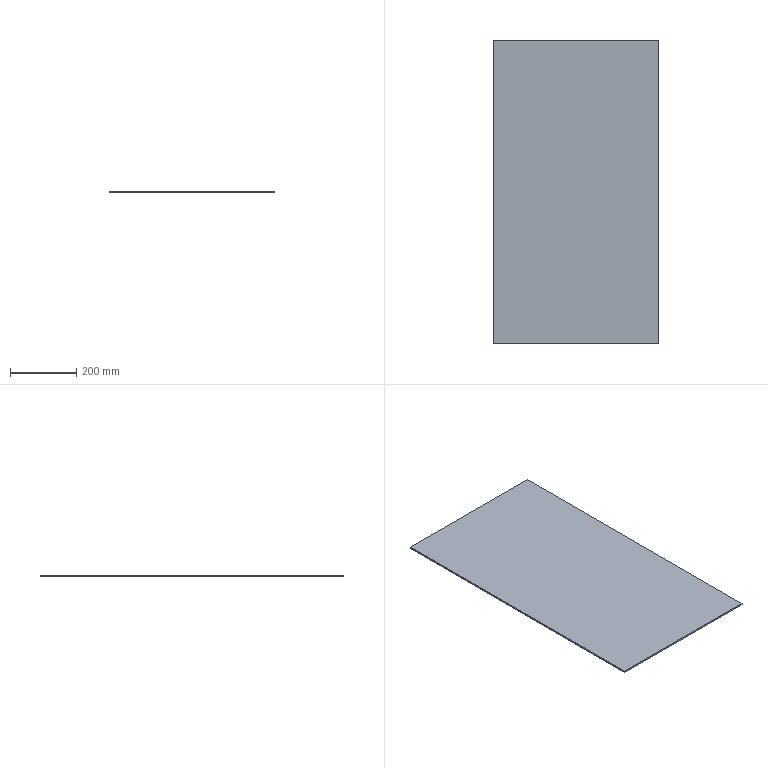Part | SolidWorks | features Extrusion 1, HoleWzd 1 | 1 solid | 6 faces | box 499 x 916 x 5 mm | volume 2285420 mm3 | plane 6
STEP:
#1=CARTESIAN_POINT('',(249.5,-458.,0.));
#2=VERTEX_POINT('',#1);
#3=CARTESIAN_POINT('',(249.5,458.,0.));
#4=VERTEX_POINT('',#3);
#5=CARTESIAN_POINT('',(249.5,458.,0.));
#6=DIRECTION('',(0.,1.,0.));
#7=VECTOR('',#6,1000.);
#8=LINE('',#5,#7);
#9=EDGE_CURVE('',#2,#4,#8,.T.);
#10=ORIENTED_EDGE('',*,*,#9,.T.);
#11=CARTESIAN_POINT('',(249.5,458.,5.));
#12=VERTEX_POINT('',#11);
#13=CARTESIAN_POINT('',(249.5,458.,5.));
#14=DIRECTION('',(0.,0.,-1.));
#15=VECTOR('',#14,1000.);
#16=LINE('',#13,#15);
#17=EDGE_CURVE('',#12,#4,#16,.T.);
#18=ORIENTED_EDGE('',*,*,#17,.F.);
#19=CARTESIAN_POINT('',(249.5,-458.,5.));
#20=VERTEX_POINT('',#19);
#21=CARTESIAN_POINT('',(249.5,458.,5.));
#22=DIRECTION('',(0.,1.,0.));
#23=VECTOR('',#22,1000.);
#24=LINE('',#21,#23);
#25=EDGE_CURVE('',#20,#12,#24,.T.);
#26=ORIENTED_EDGE('',*,*,#25,.F.);
#27=CARTESIAN_POINT('',(249.5,-458.,5.));
#28=DIRECTION('',(0.,0.,-1.));
#29=VECTOR('',#28,1000.);
#30=LINE('',#27,#29);
#31=EDGE_CURVE('',#20,#2,#30,.T.);
#32=ORIENTED_EDGE('',*,*,#31,.T.);
#33=EDGE_LOOP('',(#10,#18,#26,#32));
#34=FACE_OUTER_BOUND('',#33,.T.);
#35=CARTESIAN_POINT('',(249.5,458.,5.));
#36=DIRECTION('',(-1.,0.,0.));
#37=DIRECTION('',(0.,-1.,0.));
#38=AXIS2_PLACEMENT_3D('',#35,#36,#37);
#39=PLANE('',#38);
#40=ADVANCED_FACE('',(#34),#39,.F.);
#41=CARTESIAN_POINT('',(-249.5,458.,0.));
#42=VERTEX_POINT('',#41);
#43=CARTESIAN_POINT('',(-249.5,458.,0.));
#44=DIRECTION('',(-1.,0.,0.));
#45=VECTOR('',#44,1000.);
#46=LINE('',#43,#45);
#47=EDGE_CURVE('',#4,#42,#46,.T.);
#48=ORIENTED_EDGE('',*,*,#47,.T.);
#49=CARTESIAN_POINT('',(-249.5,458.,5.));
#50=VERTEX_POINT('',#49);
#51=CARTESIAN_POINT('',(-249.5,458.,5.));
#52=DIRECTION('',(0.,0.,-1.));
#53=VECTOR('',#52,1000.);
#54=LINE('',#51,#53);
#55=EDGE_CURVE('',#50,#42,#54,.T.);
#56=ORIENTED_EDGE('',*,*,#55,.F.);
#57=CARTESIAN_POINT('',(-249.5,458.,5.));
#58=DIRECTION('',(-1.,0.,0.));
#59=VECTOR('',#58,1000.);
#60=LINE('',#57,#59);
#61=EDGE_CURVE('',#12,#50,#60,.T.);
#62=ORIENTED_EDGE('',*,*,#61,.F.);
#63=ORIENTED_EDGE('',*,*,#17,.T.);
#64=EDGE_LOOP('',(#48,#56,#62,#63));
#65=FACE_OUTER_BOUND('',#64,.T.);
#66=CARTESIAN_POINT('',(-249.5,458.,5.));
#67=DIRECTION('',(0.,-1.,0.));
#68=DIRECTION('',(0.,0.,-1.));
#69=AXIS2_PLACEMENT_3D('',#66,#67,#68);
#70=PLANE('',#69);
#71=ADVANCED_FACE('',(#65),#70,.F.);
#72=CARTESIAN_POINT('',(-249.5,-458.,0.));
#73=VERTEX_POINT('',#72);
#74=CARTESIAN_POINT('',(-249.5,458.,0.));
#75=DIRECTION('',(0.,-1.,0.));
#76=VECTOR('',#75,1000.);
#77=LINE('',#74,#76);
#78=EDGE_CURVE('',#42,#73,#77,.T.);
#79=ORIENTED_EDGE('',*,*,#78,.T.);
#80=CARTESIAN_POINT('',(-249.5,-458.,5.));
#81=VERTEX_POINT('',#80);
#82=CARTESIAN_POINT('',(-249.5,-458.,5.));
#83=DIRECTION('',(0.,0.,-1.));
#84=VECTOR('',#83,1000.);
#85=LINE('',#82,#84);
#86=EDGE_CURVE('',#81,#73,#85,.T.);
#87=ORIENTED_EDGE('',*,*,#86,.F.);
#88=CARTESIAN_POINT('',(-249.5,458.,5.));
#89=DIRECTION('',(0.,-1.,0.));
#90=VECTOR('',#89,1000.);
#91=LINE('',#88,#90);
#92=EDGE_CURVE('',#50,#81,#91,.T.);
#93=ORIENTED_EDGE('',*,*,#92,.F.);
#94=ORIENTED_EDGE('',*,*,#55,.T.);
#95=EDGE_LOOP('',(#79,#87,#93,#94));
#96=FACE_OUTER_BOUND('',#95,.T.);
#97=CARTESIAN_POINT('',(-249.5,458.,5.));
#98=DIRECTION('',(1.,0.,0.));
#99=DIRECTION('',(0.,1.,0.));
#100=AXIS2_PLACEMENT_3D('',#97,#98,#99);
#101=PLANE('',#100);
#102=ADVANCED_FACE('',(#96),#101,.F.);
#103=CARTESIAN_POINT('',(-249.5,-458.,0.));
#104=DIRECTION('',(1.,0.,0.));
#105=VECTOR('',#104,1000.);
#106=LINE('',#103,#105);
#107=EDGE_CURVE('',#73,#2,#106,.T.);
#108=ORIENTED_EDGE('',*,*,#107,.T.);
#109=ORIENTED_EDGE('',*,*,#31,.F.);
#110=CARTESIAN_POINT('',(-249.5,-458.,5.));
#111=DIRECTION('',(1.,0.,0.));
#112=VECTOR('',#111,1000.);
#113=LINE('',#110,#112);
#114=EDGE_CURVE('',#81,#20,#113,.T.);
#115=ORIENTED_EDGE('',*,*,#114,.F.);
#116=ORIENTED_EDGE('',*,*,#86,.T.);
#117=EDGE_LOOP('',(#108,#109,#115,#116));
#118=FACE_OUTER_BOUND('',#117,.T.);
#119=CARTESIAN_POINT('',(-249.5,-458.,5.));
#120=DIRECTION('',(0.,1.,0.));
#121=DIRECTION('',(0.,0.,1.));
#122=AXIS2_PLACEMENT_3D('',#119,#120,#121);
#123=PLANE('',#122);
#124=ADVANCED_FACE('',(#118),#123,.F.);
#125=ORIENTED_EDGE('',*,*,#25,.T.);
#126=ORIENTED_EDGE('',*,*,#61,.T.);
#127=ORIENTED_EDGE('',*,*,#92,.T.);
#128=ORIENTED_EDGE('',*,*,#114,.T.);
#129=EDGE_LOOP('',(#125,#126,#127,#128));
#130=FACE_OUTER_BOUND('',#129,.T.);
#131=CARTESIAN_POINT('',(0.,0.,5.));
#132=DIRECTION('',(0.,0.,1.));
#133=DIRECTION('',(1.,0.,0.));
#134=AXIS2_PLACEMENT_3D('',#131,#132,#133);
#135=PLANE('',#134);
#136=ADVANCED_FACE('',(#130),#135,.T.);
#137=ORIENTED_EDGE('',*,*,#9,.F.);
#138=ORIENTED_EDGE('',*,*,#107,.F.);
#139=ORIENTED_EDGE('',*,*,#78,.F.);
#140=ORIENTED_EDGE('',*,*,#47,.F.);
#141=EDGE_LOOP('',(#137,#138,#139,#140));
#142=FACE_OUTER_BOUND('',#141,.T.);
#143=CARTESIAN_POINT('',(0.,0.,0.));
#144=DIRECTION('',(0.,0.,1.));
#145=DIRECTION('',(1.,0.,0.));
#146=AXIS2_PLACEMENT_3D('',#143,#144,#145);
#147=PLANE('',#146);
#148=ADVANCED_FACE('',(#142),#147,.F.);
#149=CLOSED_SHELL('',(#40,#71,#102,#124,#136,#148));
#150=MANIFOLD_SOLID_BREP('',#149);
#151=CARTESIAN_POINT('',(0.,0.,0.));
#152=DIRECTION('',(0.,0.,1.));
#153=DIRECTION('',(1.,0.,0.));
#154=AXIS2_PLACEMENT_3D('',#151,#152,#153);
#155=(LENGTH_UNIT()NAMED_UNIT(*)SI_UNIT(.MILLI.,.METRE.));
#156=UNCERTAINTY_MEASURE_WITH_UNIT(LENGTH_MEASURE(0.00001),#155,'','');
#157=(NAMED_UNIT(*)PLANE_ANGLE_UNIT()SI_UNIT($,.RADIAN.));
#158=(NAMED_UNIT(*)SI_UNIT($,.STERADIAN.)SOLID_ANGLE_UNIT());
#159=(GEOMETRIC_REPRESENTATION_CONTEXT(3)GLOBAL_UNCERTAINTY_ASSIGNED_CONTEXT((#156))GLOBAL_UNIT_ASSIGNED_CONTEXT((#155,#157,#158))REPRESENTATION_CONTEXT('',''));
#160=ADVANCED_BREP_SHAPE_REPRESENTATION('',(#150,#154),#159);